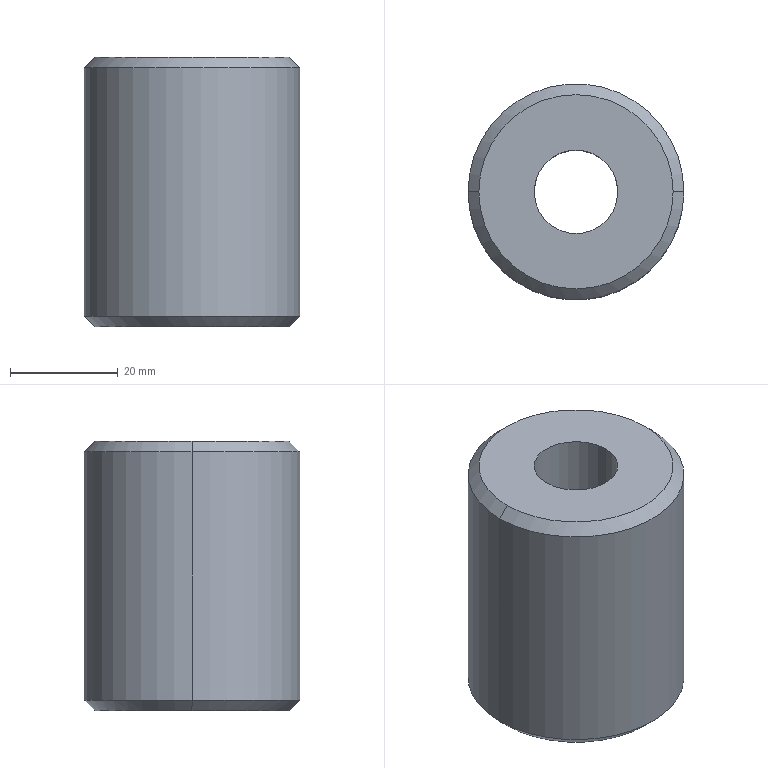Part | SolidWorks | features Chamfer 1, Extrusion 1, HoleWzd 1 | 1 solid | 10 faces | box 40 x 40 x 50 mm | volume 52911 mm3 | cylinder 4 | cone 4 | plane 2 | commonest cylinder face diameters 15.5 x2 40 x2
STEP:
#1=CARTESIAN_POINT('',(-7.75,0.,-25.));
#2=VERTEX_POINT('',#1);
#3=CARTESIAN_POINT('',(7.75,0.,-25.));
#4=VERTEX_POINT('',#3);
#5=CARTESIAN_POINT('',(0.,0.,-25.));
#6=DIRECTION('',(0.,0.,1.));
#7=DIRECTION('',(1.,0.,0.));
#8=AXIS2_PLACEMENT_3D('',#5,#6,#7);
#9=CIRCLE('',#8,7.75);
#10=EDGE_CURVE('',#2,#4,#9,.T.);
#11=ORIENTED_EDGE('',*,*,#10,.F.);
#12=CARTESIAN_POINT('',(-7.75,0.,25.));
#13=VERTEX_POINT('',#12);
#14=CARTESIAN_POINT('',(-7.75,0.,25.));
#15=DIRECTION('',(0.,0.,1.));
#16=VECTOR('',#15,1000.);
#17=LINE('',#14,#16);
#18=EDGE_CURVE('',#2,#13,#17,.T.);
#19=ORIENTED_EDGE('',*,*,#18,.T.);
#20=CARTESIAN_POINT('',(7.75,0.,25.));
#21=VERTEX_POINT('',#20);
#22=CARTESIAN_POINT('',(0.,0.,25.));
#23=DIRECTION('',(0.,0.,1.));
#24=DIRECTION('',(1.,0.,0.));
#25=AXIS2_PLACEMENT_3D('',#22,#23,#24);
#26=CIRCLE('',#25,7.75);
#27=EDGE_CURVE('',#13,#21,#26,.T.);
#28=ORIENTED_EDGE('',*,*,#27,.T.);
#29=CARTESIAN_POINT('',(7.75,0.,25.));
#30=DIRECTION('',(0.,0.,1.));
#31=VECTOR('',#30,1000.);
#32=LINE('',#29,#31);
#33=EDGE_CURVE('',#4,#21,#32,.T.);
#34=ORIENTED_EDGE('',*,*,#33,.F.);
#35=EDGE_LOOP('',(#11,#19,#28,#34));
#36=FACE_OUTER_BOUND('',#35,.T.);
#37=CARTESIAN_POINT('',(0.,0.,25.));
#38=DIRECTION('',(0.,0.,1.));
#39=DIRECTION('',(1.,0.,0.));
#40=AXIS2_PLACEMENT_3D('',#37,#38,#39);
#41=CYLINDRICAL_SURFACE('',#40,7.75);
#42=ADVANCED_FACE('',(#36),#41,.F.);
#43=CARTESIAN_POINT('',(18.,0.,25.));
#44=VERTEX_POINT('',#43);
#45=CARTESIAN_POINT('',(-18.,0.,25.));
#46=VERTEX_POINT('',#45);
#47=CARTESIAN_POINT('',(0.,0.,25.));
#48=DIRECTION('',(0.,0.,1.));
#49=DIRECTION('',(1.,0.,0.));
#50=AXIS2_PLACEMENT_3D('',#47,#48,#49);
#51=CIRCLE('',#50,18.);
#52=EDGE_CURVE('',#44,#46,#51,.T.);
#53=ORIENTED_EDGE('',*,*,#52,.F.);
#54=CARTESIAN_POINT('',(20.,0.,23.));
#55=VERTEX_POINT('',#54);
#56=CARTESIAN_POINT('',(18.,0.,25.));
#57=DIRECTION('',(0.7071,0.,-0.7071));
#58=VECTOR('',#57,1000.);
#59=LINE('',#56,#58);
#60=EDGE_CURVE('',#44,#55,#59,.T.);
#61=ORIENTED_EDGE('',*,*,#60,.T.);
#62=CARTESIAN_POINT('',(-20.,0.,23.));
#63=VERTEX_POINT('',#62);
#64=CARTESIAN_POINT('',(0.,0.,23.));
#65=DIRECTION('',(0.,0.,-1.));
#66=DIRECTION('',(1.,0.,0.));
#67=AXIS2_PLACEMENT_3D('',#64,#65,#66);
#68=CIRCLE('',#67,20.);
#69=EDGE_CURVE('',#63,#55,#68,.T.);
#70=ORIENTED_EDGE('',*,*,#69,.F.);
#71=CARTESIAN_POINT('',(-18.,0.,25.));
#72=DIRECTION('',(-0.7071,0.,-0.7071));
#73=VECTOR('',#72,1000.);
#74=LINE('',#71,#73);
#75=EDGE_CURVE('',#46,#63,#74,.T.);
#76=ORIENTED_EDGE('',*,*,#75,.F.);
#77=EDGE_LOOP('',(#53,#61,#70,#76));
#78=FACE_OUTER_BOUND('',#77,.T.);
#79=CARTESIAN_POINT('',(0.,0.,25.));
#80=DIRECTION('',(0.,0.,-1.));
#81=DIRECTION('',(-1.,0.,0.));
#82=AXIS2_PLACEMENT_3D('',#79,#80,#81);
#83=CONICAL_SURFACE('',#82,18.,0.7854);
#84=ADVANCED_FACE('',(#78),#83,.T.);
#85=CARTESIAN_POINT('',(-18.,0.,-25.));
#86=VERTEX_POINT('',#85);
#87=CARTESIAN_POINT('',(18.,0.,-25.));
#88=VERTEX_POINT('',#87);
#89=CARTESIAN_POINT('',(0.,0.,-25.));
#90=DIRECTION('',(0.,0.,-1.));
#91=DIRECTION('',(1.,0.,0.));
#92=AXIS2_PLACEMENT_3D('',#89,#90,#91);
#93=CIRCLE('',#92,18.);
#94=EDGE_CURVE('',#86,#88,#93,.T.);
#95=ORIENTED_EDGE('',*,*,#94,.F.);
#96=CARTESIAN_POINT('',(-20.,0.,-23.));
#97=VERTEX_POINT('',#96);
#98=CARTESIAN_POINT('',(-20.,0.,-23.));
#99=DIRECTION('',(-0.7071,0.,0.7071));
#100=VECTOR('',#99,1000.);
#101=LINE('',#98,#100);
#102=EDGE_CURVE('',#86,#97,#101,.T.);
#103=ORIENTED_EDGE('',*,*,#102,.T.);
#104=CARTESIAN_POINT('',(20.,0.,-23.));
#105=VERTEX_POINT('',#104);
#106=CARTESIAN_POINT('',(0.,0.,-23.));
#107=DIRECTION('',(0.,0.,1.));
#108=DIRECTION('',(1.,0.,0.));
#109=AXIS2_PLACEMENT_3D('',#106,#107,#108);
#110=CIRCLE('',#109,20.);
#111=EDGE_CURVE('',#105,#97,#110,.T.);
#112=ORIENTED_EDGE('',*,*,#111,.F.);
#113=CARTESIAN_POINT('',(20.,0.,-23.));
#114=DIRECTION('',(0.7071,0.,0.7071));
#115=VECTOR('',#114,1000.);
#116=LINE('',#113,#115);
#117=EDGE_CURVE('',#88,#105,#116,.T.);
#118=ORIENTED_EDGE('',*,*,#117,.F.);
#119=EDGE_LOOP('',(#95,#103,#112,#118));
#120=FACE_OUTER_BOUND('',#119,.T.);
#121=CARTESIAN_POINT('',(0.,0.,-23.));
#122=DIRECTION('',(0.,0.,1.));
#123=DIRECTION('',(1.,0.,0.));
#124=AXIS2_PLACEMENT_3D('',#121,#122,#123);
#125=CONICAL_SURFACE('',#124,20.,0.7854);
#126=ADVANCED_FACE('',(#120),#125,.T.);
#127=ORIENTED_EDGE('',*,*,#69,.T.);
#128=CARTESIAN_POINT('',(20.,0.,25.));
#129=DIRECTION('',(0.,0.,-1.));
#130=VECTOR('',#129,1000.);
#131=LINE('',#128,#130);
#132=EDGE_CURVE('',#55,#105,#131,.T.);
#133=ORIENTED_EDGE('',*,*,#132,.T.);
#134=ORIENTED_EDGE('',*,*,#111,.T.);
#135=CARTESIAN_POINT('',(-20.,0.,25.));
#136=DIRECTION('',(0.,0.,-1.));
#137=VECTOR('',#136,1000.);
#138=LINE('',#135,#137);
#139=EDGE_CURVE('',#63,#97,#138,.T.);
#140=ORIENTED_EDGE('',*,*,#139,.F.);
#141=EDGE_LOOP('',(#127,#133,#134,#140));
#142=FACE_OUTER_BOUND('',#141,.T.);
#143=CARTESIAN_POINT('',(0.,0.,25.));
#144=DIRECTION('',(0.,0.,-1.));
#145=DIRECTION('',(-1.,0.,0.));
#146=AXIS2_PLACEMENT_3D('',#143,#144,#145);
#147=CYLINDRICAL_SURFACE('',#146,20.);
#148=ADVANCED_FACE('',(#142),#147,.T.);
#149=ORIENTED_EDGE('',*,*,#132,.F.);
#150=CARTESIAN_POINT('',(0.,0.,23.));
#151=DIRECTION('',(0.,0.,-1.));
#152=DIRECTION('',(1.,0.,0.));
#153=AXIS2_PLACEMENT_3D('',#150,#151,#152);
#154=CIRCLE('',#153,20.);
#155=EDGE_CURVE('',#55,#63,#154,.T.);
#156=ORIENTED_EDGE('',*,*,#155,.T.);
#157=ORIENTED_EDGE('',*,*,#139,.T.);
#158=CARTESIAN_POINT('',(0.,0.,-23.));
#159=DIRECTION('',(0.,0.,1.));
#160=DIRECTION('',(1.,0.,0.));
#161=AXIS2_PLACEMENT_3D('',#158,#159,#160);
#162=CIRCLE('',#161,20.);
#163=EDGE_CURVE('',#97,#105,#162,.T.);
#164=ORIENTED_EDGE('',*,*,#163,.T.);
#165=EDGE_LOOP('',(#149,#156,#157,#164));
#166=FACE_OUTER_BOUND('',#165,.T.);
#167=CARTESIAN_POINT('',(0.,0.,25.));
#168=DIRECTION('',(0.,0.,-1.));
#169=DIRECTION('',(-1.,0.,0.));
#170=AXIS2_PLACEMENT_3D('',#167,#168,#169);
#171=CYLINDRICAL_SURFACE('',#170,20.);
#172=ADVANCED_FACE('',(#166),#171,.T.);
#173=CARTESIAN_POINT('',(0.,0.,25.));
#174=DIRECTION('',(0.,0.,1.));
#175=DIRECTION('',(1.,0.,0.));
#176=AXIS2_PLACEMENT_3D('',#173,#174,#175);
#177=CIRCLE('',#176,7.75);
#178=EDGE_CURVE('',#21,#13,#177,.T.);
#179=ORIENTED_EDGE('',*,*,#178,.F.);
#180=ORIENTED_EDGE('',*,*,#27,.F.);
#181=EDGE_LOOP('',(#179,#180));
#182=FACE_BOUND('',#181,.T.);
#183=CARTESIAN_POINT('',(0.,0.,25.));
#184=DIRECTION('',(0.,0.,1.));
#185=DIRECTION('',(1.,0.,0.));
#186=AXIS2_PLACEMENT_3D('',#183,#184,#185);
#187=CIRCLE('',#186,18.);
#188=EDGE_CURVE('',#46,#44,#187,.T.);
#189=ORIENTED_EDGE('',*,*,#188,.T.);
#190=ORIENTED_EDGE('',*,*,#52,.T.);
#191=EDGE_LOOP('',(#189,#190));
#192=FACE_OUTER_BOUND('',#191,.T.);
#193=CARTESIAN_POINT('',(0.,0.,25.));
#194=DIRECTION('',(0.,0.,1.));
#195=DIRECTION('',(1.,0.,0.));
#196=AXIS2_PLACEMENT_3D('',#193,#194,#195);
#197=PLANE('',#196);
#198=ADVANCED_FACE('',(#182,#192),#197,.T.);
#199=CARTESIAN_POINT('',(0.,0.,-25.));
#200=DIRECTION('',(0.,0.,1.));
#201=DIRECTION('',(1.,0.,0.));
#202=AXIS2_PLACEMENT_3D('',#199,#200,#201);
#203=CIRCLE('',#202,7.75);
#204=EDGE_CURVE('',#4,#2,#203,.T.);
#205=ORIENTED_EDGE('',*,*,#204,.T.);
#206=ORIENTED_EDGE('',*,*,#10,.T.);
#207=EDGE_LOOP('',(#205,#206));
#208=FACE_BOUND('',#207,.T.);
#209=CARTESIAN_POINT('',(0.,0.,-25.));
#210=DIRECTION('',(0.,0.,-1.));
#211=DIRECTION('',(1.,0.,0.));
#212=AXIS2_PLACEMENT_3D('',#209,#210,#211);
#213=CIRCLE('',#212,18.);
#214=EDGE_CURVE('',#88,#86,#213,.T.);
#215=ORIENTED_EDGE('',*,*,#214,.T.);
#216=ORIENTED_EDGE('',*,*,#94,.T.);
#217=EDGE_LOOP('',(#215,#216));
#218=FACE_OUTER_BOUND('',#217,.T.);
#219=CARTESIAN_POINT('',(0.,0.,-25.));
#220=DIRECTION('',(0.,0.,1.));
#221=DIRECTION('',(1.,0.,0.));
#222=AXIS2_PLACEMENT_3D('',#219,#220,#221);
#223=PLANE('',#222);
#224=ADVANCED_FACE('',(#208,#218),#223,.F.);
#225=ORIENTED_EDGE('',*,*,#102,.F.);
#226=ORIENTED_EDGE('',*,*,#214,.F.);
#227=ORIENTED_EDGE('',*,*,#117,.T.);
#228=ORIENTED_EDGE('',*,*,#163,.F.);
#229=EDGE_LOOP('',(#225,#226,#227,#228));
#230=FACE_OUTER_BOUND('',#229,.T.);
#231=CARTESIAN_POINT('',(0.,0.,-23.));
#232=DIRECTION('',(0.,0.,1.));
#233=DIRECTION('',(1.,0.,0.));
#234=AXIS2_PLACEMENT_3D('',#231,#232,#233);
#235=CONICAL_SURFACE('',#234,20.,0.7854);
#236=ADVANCED_FACE('',(#230),#235,.T.);
#237=ORIENTED_EDGE('',*,*,#60,.F.);
#238=ORIENTED_EDGE('',*,*,#188,.F.);
#239=ORIENTED_EDGE('',*,*,#75,.T.);
#240=ORIENTED_EDGE('',*,*,#155,.F.);
#241=EDGE_LOOP('',(#237,#238,#239,#240));
#242=FACE_OUTER_BOUND('',#241,.T.);
#243=CARTESIAN_POINT('',(0.,0.,25.));
#244=DIRECTION('',(0.,0.,-1.));
#245=DIRECTION('',(-1.,0.,0.));
#246=AXIS2_PLACEMENT_3D('',#243,#244,#245);
#247=CONICAL_SURFACE('',#246,18.,0.7854);
#248=ADVANCED_FACE('',(#242),#247,.T.);
#249=ORIENTED_EDGE('',*,*,#18,.F.);
#250=ORIENTED_EDGE('',*,*,#204,.F.);
#251=ORIENTED_EDGE('',*,*,#33,.T.);
#252=ORIENTED_EDGE('',*,*,#178,.T.);
#253=EDGE_LOOP('',(#249,#250,#251,#252));
#254=FACE_OUTER_BOUND('',#253,.T.);
#255=CARTESIAN_POINT('',(0.,0.,25.));
#256=DIRECTION('',(0.,0.,1.));
#257=DIRECTION('',(1.,0.,0.));
#258=AXIS2_PLACEMENT_3D('',#255,#256,#257);
#259=CYLINDRICAL_SURFACE('',#258,7.75);
#260=ADVANCED_FACE('',(#254),#259,.F.);
#261=CLOSED_SHELL('',(#42,#84,#126,#148,#172,#198,#224,#236,#248,#260));
#262=MANIFOLD_SOLID_BREP('',#261);
#263=CARTESIAN_POINT('',(0.,0.,0.));
#264=DIRECTION('',(0.,0.,1.));
#265=DIRECTION('',(1.,0.,0.));
#266=AXIS2_PLACEMENT_3D('',#263,#264,#265);
#267=(LENGTH_UNIT()NAMED_UNIT(*)SI_UNIT(.MILLI.,.METRE.));
#268=UNCERTAINTY_MEASURE_WITH_UNIT(LENGTH_MEASURE(0.00001),#267,'','');
#269=(NAMED_UNIT(*)PLANE_ANGLE_UNIT()SI_UNIT($,.RADIAN.));
#270=(NAMED_UNIT(*)SI_UNIT($,.STERADIAN.)SOLID_ANGLE_UNIT());
#271=(GEOMETRIC_REPRESENTATION_CONTEXT(3)GLOBAL_UNCERTAINTY_ASSIGNED_CONTEXT((#268))GLOBAL_UNIT_ASSIGNED_CONTEXT((#267,#269,#270))REPRESENTATION_CONTEXT('',''));
#272=ADVANCED_BREP_SHAPE_REPRESENTATION('',(#262,#266),#271);